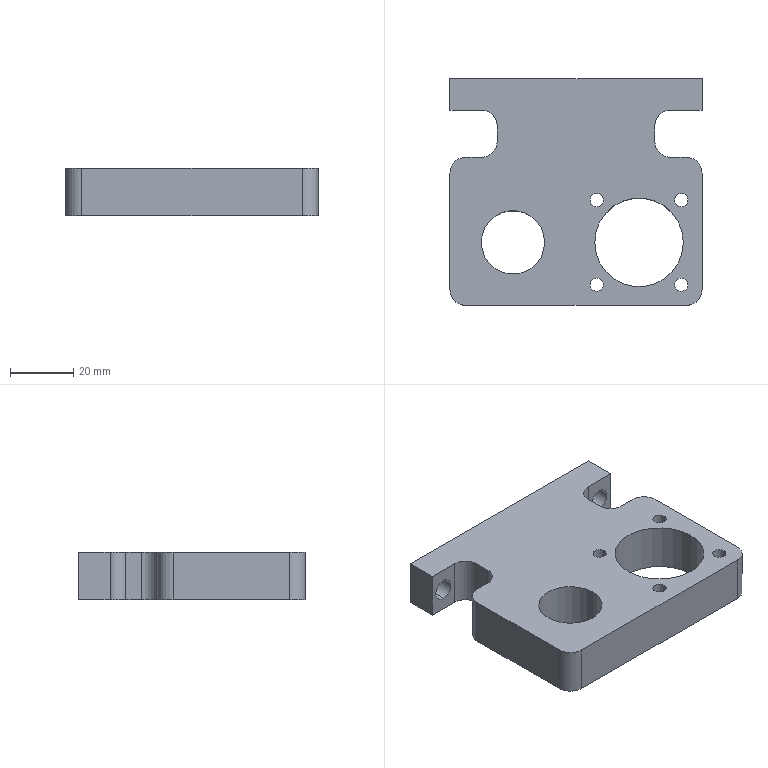Part | SolidWorks | features ICE 2, Extrusion 1, Fillet 1, HoleWzd 1, MoveCopyBody 1 | 1 solid | 38 faces | box 80 x 72 x 15 mm | volume 64030 mm3 | cylinder 24 | plane 14 | commonest cylinder face diameters 4.2 x8 10 x8 6.8 x4 20.1 x2 28.1 x2
STEP:
#1=CARTESIAN_POINT('',(31.335,21.435,7.5));
#2=VERTEX_POINT('',#1);
#3=CARTESIAN_POINT('',(35.535,21.435,7.5));
#4=VERTEX_POINT('',#3);
#5=CARTESIAN_POINT('',(33.435,21.435,7.5));
#6=DIRECTION('',(0.,0.,-1.));
#7=DIRECTION('',(1.,0.,0.));
#8=AXIS2_PLACEMENT_3D('',#5,#6,#7);
#9=CIRCLE('',#8,2.1);
#10=EDGE_CURVE('',#2,#4,#9,.T.);
#11=ORIENTED_EDGE('',*,*,#10,.F.);
#12=CARTESIAN_POINT('',(31.335,21.435,-7.5));
#13=VERTEX_POINT('',#12);
#14=CARTESIAN_POINT('',(31.335,21.435,-7.5));
#15=DIRECTION('',(0.,0.,-1.));
#16=VECTOR('',#15,1000.);
#17=LINE('',#14,#16);
#18=EDGE_CURVE('',#2,#13,#17,.T.);
#19=ORIENTED_EDGE('',*,*,#18,.T.);
#20=CARTESIAN_POINT('',(35.535,21.435,-7.5));
#21=VERTEX_POINT('',#20);
#22=CARTESIAN_POINT('',(33.435,21.435,-7.5));
#23=DIRECTION('',(0.,0.,-1.));
#24=DIRECTION('',(1.,0.,0.));
#25=AXIS2_PLACEMENT_3D('',#22,#23,#24);
#26=CIRCLE('',#25,2.1);
#27=EDGE_CURVE('',#13,#21,#26,.T.);
#28=ORIENTED_EDGE('',*,*,#27,.T.);
#29=CARTESIAN_POINT('',(35.535,21.435,-7.5));
#30=DIRECTION('',(0.,0.,-1.));
#31=VECTOR('',#30,1000.);
#32=LINE('',#29,#31);
#33=EDGE_CURVE('',#4,#21,#32,.T.);
#34=ORIENTED_EDGE('',*,*,#33,.F.);
#35=EDGE_LOOP('',(#11,#19,#28,#34));
#36=FACE_OUTER_BOUND('',#35,.T.);
#37=CARTESIAN_POINT('',(33.435,21.435,-7.5));
#38=DIRECTION('',(0.,0.,-1.));
#39=DIRECTION('',(1.,0.,0.));
#40=AXIS2_PLACEMENT_3D('',#37,#38,#39);
#41=CYLINDRICAL_SURFACE('',#40,2.1);
#42=ADVANCED_FACE('',(#36),#41,.F.);
#43=CARTESIAN_POINT('',(4.465,21.435,7.5));
#44=VERTEX_POINT('',#43);
#45=CARTESIAN_POINT('',(8.665,21.435,7.5));
#46=VERTEX_POINT('',#45);
#47=CARTESIAN_POINT('',(6.565,21.435,7.5));
#48=DIRECTION('',(0.,0.,-1.));
#49=DIRECTION('',(1.,0.,0.));
#50=AXIS2_PLACEMENT_3D('',#47,#48,#49);
#51=CIRCLE('',#50,2.1);
#52=EDGE_CURVE('',#44,#46,#51,.T.);
#53=ORIENTED_EDGE('',*,*,#52,.F.);
#54=CARTESIAN_POINT('',(4.465,21.435,-7.5));
#55=VERTEX_POINT('',#54);
#56=CARTESIAN_POINT('',(4.465,21.435,-7.5));
#57=DIRECTION('',(0.,0.,-1.));
#58=VECTOR('',#57,1000.);
#59=LINE('',#56,#58);
#60=EDGE_CURVE('',#44,#55,#59,.T.);
#61=ORIENTED_EDGE('',*,*,#60,.T.);
#62=CARTESIAN_POINT('',(8.665,21.435,-7.5));
#63=VERTEX_POINT('',#62);
#64=CARTESIAN_POINT('',(6.565,21.435,-7.5));
#65=DIRECTION('',(0.,0.,-1.));
#66=DIRECTION('',(1.,0.,0.));
#67=AXIS2_PLACEMENT_3D('',#64,#65,#66);
#68=CIRCLE('',#67,2.1);
#69=EDGE_CURVE('',#55,#63,#68,.T.);
#70=ORIENTED_EDGE('',*,*,#69,.T.);
#71=CARTESIAN_POINT('',(8.665,21.435,-7.5));
#72=DIRECTION('',(0.,0.,-1.));
#73=VECTOR('',#72,1000.);
#74=LINE('',#71,#73);
#75=EDGE_CURVE('',#46,#63,#74,.T.);
#76=ORIENTED_EDGE('',*,*,#75,.F.);
#77=EDGE_LOOP('',(#53,#61,#70,#76));
#78=FACE_OUTER_BOUND('',#77,.T.);
#79=CARTESIAN_POINT('',(6.565,21.435,-7.5));
#80=DIRECTION('',(0.,0.,-1.));
#81=DIRECTION('',(1.,0.,0.));
#82=AXIS2_PLACEMENT_3D('',#79,#80,#81);
#83=CYLINDRICAL_SURFACE('',#82,2.1);
#84=ADVANCED_FACE('',(#78),#83,.F.);
#85=CARTESIAN_POINT('',(4.465,-5.435,7.5));
#86=VERTEX_POINT('',#85);
#87=CARTESIAN_POINT('',(8.665,-5.435,7.5));
#88=VERTEX_POINT('',#87);
#89=CARTESIAN_POINT('',(6.565,-5.435,7.5));
#90=DIRECTION('',(0.,0.,-1.));
#91=DIRECTION('',(1.,0.,0.));
#92=AXIS2_PLACEMENT_3D('',#89,#90,#91);
#93=CIRCLE('',#92,2.1);
#94=EDGE_CURVE('',#86,#88,#93,.T.);
#95=ORIENTED_EDGE('',*,*,#94,.F.);
#96=CARTESIAN_POINT('',(4.465,-5.435,-7.5));
#97=VERTEX_POINT('',#96);
#98=CARTESIAN_POINT('',(4.465,-5.435,-7.5));
#99=DIRECTION('',(0.,0.,-1.));
#100=VECTOR('',#99,1000.);
#101=LINE('',#98,#100);
#102=EDGE_CURVE('',#86,#97,#101,.T.);
#103=ORIENTED_EDGE('',*,*,#102,.T.);
#104=CARTESIAN_POINT('',(8.665,-5.435,-7.5));
#105=VERTEX_POINT('',#104);
#106=CARTESIAN_POINT('',(6.565,-5.435,-7.5));
#107=DIRECTION('',(0.,0.,-1.));
#108=DIRECTION('',(1.,0.,0.));
#109=AXIS2_PLACEMENT_3D('',#106,#107,#108);
#110=CIRCLE('',#109,2.1);
#111=EDGE_CURVE('',#97,#105,#110,.T.);
#112=ORIENTED_EDGE('',*,*,#111,.T.);
#113=CARTESIAN_POINT('',(8.665,-5.435,-7.5));
#114=DIRECTION('',(0.,0.,-1.));
#115=VECTOR('',#114,1000.);
#116=LINE('',#113,#115);
#117=EDGE_CURVE('',#88,#105,#116,.T.);
#118=ORIENTED_EDGE('',*,*,#117,.F.);
#119=EDGE_LOOP('',(#95,#103,#112,#118));
#120=FACE_OUTER_BOUND('',#119,.T.);
#121=CARTESIAN_POINT('',(6.565,-5.435,-7.5));
#122=DIRECTION('',(0.,0.,-1.));
#123=DIRECTION('',(1.,0.,0.));
#124=AXIS2_PLACEMENT_3D('',#121,#122,#123);
#125=CYLINDRICAL_SURFACE('',#124,2.1);
#126=ADVANCED_FACE('',(#120),#125,.F.);
#127=CARTESIAN_POINT('',(31.335,-5.435,7.5));
#128=VERTEX_POINT('',#127);
#129=CARTESIAN_POINT('',(35.535,-5.435,7.5));
#130=VERTEX_POINT('',#129);
#131=CARTESIAN_POINT('',(33.435,-5.435,7.5));
#132=DIRECTION('',(0.,0.,-1.));
#133=DIRECTION('',(1.,0.,0.));
#134=AXIS2_PLACEMENT_3D('',#131,#132,#133);
#135=CIRCLE('',#134,2.1);
#136=EDGE_CURVE('',#128,#130,#135,.T.);
#137=ORIENTED_EDGE('',*,*,#136,.F.);
#138=CARTESIAN_POINT('',(31.335,-5.435,-7.5));
#139=VERTEX_POINT('',#138);
#140=CARTESIAN_POINT('',(31.335,-5.435,-7.5));
#141=DIRECTION('',(0.,0.,-1.));
#142=VECTOR('',#141,1000.);
#143=LINE('',#140,#142);
#144=EDGE_CURVE('',#128,#139,#143,.T.);
#145=ORIENTED_EDGE('',*,*,#144,.T.);
#146=CARTESIAN_POINT('',(35.535,-5.435,-7.5));
#147=VERTEX_POINT('',#146);
#148=CARTESIAN_POINT('',(33.435,-5.435,-7.5));
#149=DIRECTION('',(0.,0.,-1.));
#150=DIRECTION('',(1.,0.,0.));
#151=AXIS2_PLACEMENT_3D('',#148,#149,#150);
#152=CIRCLE('',#151,2.1);
#153=EDGE_CURVE('',#139,#147,#152,.T.);
#154=ORIENTED_EDGE('',*,*,#153,.T.);
#155=CARTESIAN_POINT('',(35.535,-5.435,-7.5));
#156=DIRECTION('',(0.,0.,-1.));
#157=VECTOR('',#156,1000.);
#158=LINE('',#155,#157);
#159=EDGE_CURVE('',#130,#147,#158,.T.);
#160=ORIENTED_EDGE('',*,*,#159,.F.);
#161=EDGE_LOOP('',(#137,#145,#154,#160));
#162=FACE_OUTER_BOUND('',#161,.T.);
#163=CARTESIAN_POINT('',(33.435,-5.435,-7.5));
#164=DIRECTION('',(0.,0.,-1.));
#165=DIRECTION('',(1.,0.,0.));
#166=AXIS2_PLACEMENT_3D('',#163,#164,#165);
#167=CYLINDRICAL_SURFACE('',#166,2.1);
#168=ADVANCED_FACE('',(#162),#167,.F.);
#169=CARTESIAN_POINT('',(34.05,8.,-7.5));
#170=VERTEX_POINT('',#169);
#171=CARTESIAN_POINT('',(5.95,8.,-7.5));
#172=VERTEX_POINT('',#171);
#173=CARTESIAN_POINT('',(20.,8.,-7.5));
#174=DIRECTION('',(0.,0.,1.));
#175=DIRECTION('',(-1.,0.,0.));
#176=AXIS2_PLACEMENT_3D('',#173,#174,#175);
#177=CIRCLE('',#176,14.05);
#178=EDGE_CURVE('',#170,#172,#177,.T.);
#179=ORIENTED_EDGE('',*,*,#178,.F.);
#180=CARTESIAN_POINT('',(34.05,8.,7.5));
#181=VERTEX_POINT('',#180);
#182=CARTESIAN_POINT('',(34.05,8.,-7.5));
#183=DIRECTION('',(0.,0.,1.));
#184=VECTOR('',#183,1000.);
#185=LINE('',#182,#184);
#186=EDGE_CURVE('',#170,#181,#185,.T.);
#187=ORIENTED_EDGE('',*,*,#186,.T.);
#188=CARTESIAN_POINT('',(5.95,8.,7.5));
#189=VERTEX_POINT('',#188);
#190=CARTESIAN_POINT('',(20.,8.,7.5));
#191=DIRECTION('',(0.,0.,1.));
#192=DIRECTION('',(-1.,0.,0.));
#193=AXIS2_PLACEMENT_3D('',#190,#191,#192);
#194=CIRCLE('',#193,14.05);
#195=EDGE_CURVE('',#181,#189,#194,.T.);
#196=ORIENTED_EDGE('',*,*,#195,.T.);
#197=CARTESIAN_POINT('',(5.95,8.,-7.5));
#198=DIRECTION('',(0.,0.,1.));
#199=VECTOR('',#198,1000.);
#200=LINE('',#197,#199);
#201=EDGE_CURVE('',#172,#189,#200,.T.);
#202=ORIENTED_EDGE('',*,*,#201,.F.);
#203=EDGE_LOOP('',(#179,#187,#196,#202));
#204=FACE_OUTER_BOUND('',#203,.T.);
#205=CARTESIAN_POINT('',(20.,8.,-7.5));
#206=DIRECTION('',(0.,0.,1.));
#207=DIRECTION('',(-1.,0.,0.));
#208=AXIS2_PLACEMENT_3D('',#205,#206,#207);
#209=CYLINDRICAL_SURFACE('',#208,14.05);
#210=ADVANCED_FACE('',(#204),#209,.F.);
#211=CARTESIAN_POINT('',(-9.95,8.,-7.5));
#212=VERTEX_POINT('',#211);
#213=CARTESIAN_POINT('',(-30.05,8.,-7.5));
#214=VERTEX_POINT('',#213);
#215=CARTESIAN_POINT('',(-20.,8.,-7.5));
#216=DIRECTION('',(0.,0.,1.));
#217=DIRECTION('',(-1.,0.,0.));
#218=AXIS2_PLACEMENT_3D('',#215,#216,#217);
#219=CIRCLE('',#218,10.05);
#220=EDGE_CURVE('',#212,#214,#219,.T.);
#221=ORIENTED_EDGE('',*,*,#220,.F.);
#222=CARTESIAN_POINT('',(-9.95,8.,7.5));
#223=VERTEX_POINT('',#222);
#224=CARTESIAN_POINT('',(-9.95,8.,-7.5));
#225=DIRECTION('',(0.,0.,1.));
#226=VECTOR('',#225,1000.);
#227=LINE('',#224,#226);
#228=EDGE_CURVE('',#212,#223,#227,.T.);
#229=ORIENTED_EDGE('',*,*,#228,.T.);
#230=CARTESIAN_POINT('',(-30.05,8.,7.5));
#231=VERTEX_POINT('',#230);
#232=CARTESIAN_POINT('',(-20.,8.,7.5));
#233=DIRECTION('',(0.,0.,1.));
#234=DIRECTION('',(-1.,0.,0.));
#235=AXIS2_PLACEMENT_3D('',#232,#233,#234);
#236=CIRCLE('',#235,10.05);
#237=EDGE_CURVE('',#223,#231,#236,.T.);
#238=ORIENTED_EDGE('',*,*,#237,.T.);
#239=CARTESIAN_POINT('',(-30.05,8.,-7.5));
#240=DIRECTION('',(0.,0.,1.));
#241=VECTOR('',#240,1000.);
#242=LINE('',#239,#241);
#243=EDGE_CURVE('',#214,#231,#242,.T.);
#244=ORIENTED_EDGE('',*,*,#243,.F.);
#245=EDGE_LOOP('',(#221,#229,#238,#244));
#246=FACE_OUTER_BOUND('',#245,.T.);
#247=CARTESIAN_POINT('',(-20.,8.,-7.5));
#248=DIRECTION('',(0.,0.,1.));
#249=DIRECTION('',(-1.,0.,0.));
#250=AXIS2_PLACEMENT_3D('',#247,#248,#249);
#251=CYLINDRICAL_SURFACE('',#250,10.05);
#252=ADVANCED_FACE('',(#246),#251,.F.);
#253=CARTESIAN_POINT('',(-35.,50.,-3.4));
#254=VERTEX_POINT('',#253);
#255=CARTESIAN_POINT('',(-35.,50.,3.4));
#256=VERTEX_POINT('',#255);
#257=CARTESIAN_POINT('',(-35.,50.,0.));
#258=DIRECTION('',(0.,-1.,0.));
#259=DIRECTION('',(0.,0.,-1.));
#260=AXIS2_PLACEMENT_3D('',#257,#258,#259);
#261=CIRCLE('',#260,3.4);
#262=EDGE_CURVE('',#254,#256,#261,.T.);
#263=ORIENTED_EDGE('',*,*,#262,.T.);
#264=CARTESIAN_POINT('',(-35.,60.,3.4));
#265=VERTEX_POINT('',#264);
#266=CARTESIAN_POINT('',(-35.,-12.001,3.4));
#267=DIRECTION('',(0.,1.,0.));
#268=VECTOR('',#267,1000.);
#269=LINE('',#266,#268);
#270=EDGE_CURVE('',#256,#265,#269,.T.);
#271=ORIENTED_EDGE('',*,*,#270,.T.);
#272=CARTESIAN_POINT('',(-35.,60.,-3.4));
#273=VERTEX_POINT('',#272);
#274=CARTESIAN_POINT('',(-35.,60.,0.));
#275=DIRECTION('',(0.,1.,0.));
#276=DIRECTION('',(0.,0.,1.));
#277=AXIS2_PLACEMENT_3D('',#274,#275,#276);
#278=CIRCLE('',#277,3.4);
#279=EDGE_CURVE('',#265,#273,#278,.T.);
#280=ORIENTED_EDGE('',*,*,#279,.T.);
#281=CARTESIAN_POINT('',(-35.,-12.001,-3.4));
#282=DIRECTION('',(0.,1.,0.));
#283=VECTOR('',#282,1000.);
#284=LINE('',#281,#283);
#285=EDGE_CURVE('',#254,#273,#284,.T.);
#286=ORIENTED_EDGE('',*,*,#285,.F.);
#287=EDGE_LOOP('',(#263,#271,#280,#286));
#288=FACE_OUTER_BOUND('',#287,.T.);
#289=CARTESIAN_POINT('',(-35.,-12.001,0.));
#290=DIRECTION('',(0.,1.,0.));
#291=DIRECTION('',(0.,0.,-1.));
#292=AXIS2_PLACEMENT_3D('',#289,#290,#291);
#293=CYLINDRICAL_SURFACE('',#292,3.4);
#294=ADVANCED_FACE('',(#288),#293,.F.);
#295=CARTESIAN_POINT('',(35.,50.,-3.4));
#296=VERTEX_POINT('',#295);
#297=CARTESIAN_POINT('',(35.,50.,3.4));
#298=VERTEX_POINT('',#297);
#299=CARTESIAN_POINT('',(35.,50.,0.));
#300=DIRECTION('',(0.,-1.,0.));
#301=DIRECTION('',(0.,0.,-1.));
#302=AXIS2_PLACEMENT_3D('',#299,#300,#301);
#303=CIRCLE('',#302,3.4);
#304=EDGE_CURVE('',#296,#298,#303,.T.);
#305=ORIENTED_EDGE('',*,*,#304,.T.);
#306=CARTESIAN_POINT('',(35.,60.,3.4));
#307=VERTEX_POINT('',#306);
#308=CARTESIAN_POINT('',(35.,-12.001,3.4));
#309=DIRECTION('',(0.,1.,0.));
#310=VECTOR('',#309,1000.);
#311=LINE('',#308,#310);
#312=EDGE_CURVE('',#298,#307,#311,.T.);
#313=ORIENTED_EDGE('',*,*,#312,.T.);
#314=CARTESIAN_POINT('',(35.,60.,-3.4));
#315=VERTEX_POINT('',#314);
#316=CARTESIAN_POINT('',(35.,60.,0.));
#317=DIRECTION('',(0.,1.,0.));
#318=DIRECTION('',(0.,0.,-1.));
#319=AXIS2_PLACEMENT_3D('',#316,#317,#318);
#320=CIRCLE('',#319,3.4);
#321=EDGE_CURVE('',#307,#315,#320,.T.);
#322=ORIENTED_EDGE('',*,*,#321,.T.);
#323=CARTESIAN_POINT('',(35.,-12.001,-3.4));
#324=DIRECTION('',(0.,1.,0.));
#325=VECTOR('',#324,1000.);
#326=LINE('',#323,#325);
#327=EDGE_CURVE('',#296,#315,#326,.T.);
#328=ORIENTED_EDGE('',*,*,#327,.F.);
#329=EDGE_LOOP('',(#305,#313,#322,#328));
#330=FACE_OUTER_BOUND('',#329,.T.);
#331=CARTESIAN_POINT('',(35.,-12.001,0.));
#332=DIRECTION('',(0.,1.,0.));
#333=DIRECTION('',(0.,0.,-1.));
#334=AXIS2_PLACEMENT_3D('',#331,#332,#333);
#335=CYLINDRICAL_SURFACE('',#334,3.4);
#336=ADVANCED_FACE('',(#330),#335,.F.);
#337=CARTESIAN_POINT('',(40.,50.,-7.5));
#338=VERTEX_POINT('',#337);
#339=CARTESIAN_POINT('',(40.,60.,-7.5));
#340=VERTEX_POINT('',#339);
#341=CARTESIAN_POINT('',(40.,60.,-7.5));
#342=DIRECTION('',(0.,1.,0.));
#343=VECTOR('',#342,1000.);
#344=LINE('',#341,#343);
#345=EDGE_CURVE('',#338,#340,#344,.T.);
#346=ORIENTED_EDGE('',*,*,#345,.T.);
#347=CARTESIAN_POINT('',(40.,60.,7.5));
#348=VERTEX_POINT('',#347);
#349=CARTESIAN_POINT('',(40.,60.,7.5));
#350=DIRECTION('',(0.,0.,-1.));
#351=VECTOR('',#350,1000.);
#352=LINE('',#349,#351);
#353=EDGE_CURVE('',#348,#340,#352,.T.);
#354=ORIENTED_EDGE('',*,*,#353,.F.);
#355=CARTESIAN_POINT('',(40.,50.,7.5));
#356=VERTEX_POINT('',#355);
#357=CARTESIAN_POINT('',(40.,60.,7.5));
#358=DIRECTION('',(0.,1.,0.));
#359=VECTOR('',#358,1000.);
#360=LINE('',#357,#359);
#361=EDGE_CURVE('',#356,#348,#360,.T.);
#362=ORIENTED_EDGE('',*,*,#361,.F.);
#363=CARTESIAN_POINT('',(40.,50.,7.5));
#364=DIRECTION('',(0.,0.,-1.));
#365=VECTOR('',#364,1000.);
#366=LINE('',#363,#365);
#367=EDGE_CURVE('',#356,#338,#366,.T.);
#368=ORIENTED_EDGE('',*,*,#367,.T.);
#369=EDGE_LOOP('',(#346,#354,#362,#368));
#370=FACE_OUTER_BOUND('',#369,.T.);
#371=CARTESIAN_POINT('',(40.,60.,7.5));
#372=DIRECTION('',(-1.,0.,0.));
#373=DIRECTION('',(0.,0.,-1.));
#374=AXIS2_PLACEMENT_3D('',#371,#372,#373);
#375=PLANE('',#374);
#376=ADVANCED_FACE('',(#370),#375,.F.);
#377=CARTESIAN_POINT('',(35.,60.,0.));
#378=DIRECTION('',(0.,1.,0.));
#379=DIRECTION('',(0.,0.,-1.));
#380=AXIS2_PLACEMENT_3D('',#377,#378,#379);
#381=CIRCLE('',#380,3.4);
#382=EDGE_CURVE('',#315,#307,#381,.T.);
#383=ORIENTED_EDGE('',*,*,#382,.F.);
#384=ORIENTED_EDGE('',*,*,#321,.F.);
#385=EDGE_LOOP('',(#383,#384));
#386=FACE_BOUND('',#385,.T.);
#387=CARTESIAN_POINT('',(-35.,60.,0.));
#388=DIRECTION('',(0.,1.,0.));
#389=DIRECTION('',(0.,0.,1.));
#390=AXIS2_PLACEMENT_3D('',#387,#388,#389);
#391=CIRCLE('',#390,3.4);
#392=EDGE_CURVE('',#273,#265,#391,.T.);
#393=ORIENTED_EDGE('',*,*,#392,.F.);
#394=ORIENTED_EDGE('',*,*,#279,.F.);
#395=EDGE_LOOP('',(#393,#394));
#396=FACE_BOUND('',#395,.T.);
#397=CARTESIAN_POINT('',(-40.,60.,-7.5));
#398=VERTEX_POINT('',#397);
#399=CARTESIAN_POINT('',(-40.,60.,-7.5));
#400=DIRECTION('',(-1.,0.,0.));
#401=VECTOR('',#400,1000.);
#402=LINE('',#399,#401);
#403=EDGE_CURVE('',#340,#398,#402,.T.);
#404=ORIENTED_EDGE('',*,*,#403,.T.);
#405=CARTESIAN_POINT('',(-40.,60.,7.5));
#406=VERTEX_POINT('',#405);
#407=CARTESIAN_POINT('',(-40.,60.,7.5));
#408=DIRECTION('',(0.,0.,-1.));
#409=VECTOR('',#408,1000.);
#410=LINE('',#407,#409);
#411=EDGE_CURVE('',#406,#398,#410,.T.);
#412=ORIENTED_EDGE('',*,*,#411,.F.);
#413=CARTESIAN_POINT('',(-40.,60.,7.5));
#414=DIRECTION('',(-1.,0.,0.));
#415=VECTOR('',#414,1000.);
#416=LINE('',#413,#415);
#417=EDGE_CURVE('',#348,#406,#416,.T.);
#418=ORIENTED_EDGE('',*,*,#417,.F.);
#419=ORIENTED_EDGE('',*,*,#353,.T.);
#420=EDGE_LOOP('',(#404,#412,#418,#419));
#421=FACE_OUTER_BOUND('',#420,.T.);
#422=CARTESIAN_POINT('',(-40.,60.,7.5));
#423=DIRECTION('',(0.,-1.,0.));
#424=DIRECTION('',(0.,0.,1.));
#425=AXIS2_PLACEMENT_3D('',#422,#423,#424);
#426=PLANE('',#425);
#427=ADVANCED_FACE('',(#386,#396,#421),#426,.F.);
#428=CARTESIAN_POINT('',(-40.,50.,-7.5));
#429=VERTEX_POINT('',#428);
#430=CARTESIAN_POINT('',(-40.,60.,-7.5));
#431=DIRECTION('',(0.,-1.,0.));
#432=VECTOR('',#431,1000.);
#433=LINE('',#430,#432);
#434=EDGE_CURVE('',#398,#429,#433,.T.);
#435=ORIENTED_EDGE('',*,*,#434,.T.);
#436=CARTESIAN_POINT('',(-40.,50.,7.5));
#437=VERTEX_POINT('',#436);
#438=CARTESIAN_POINT('',(-40.,50.,7.5));
#439=DIRECTION('',(0.,0.,-1.));
#440=VECTOR('',#439,1000.);
#441=LINE('',#438,#440);
#442=EDGE_CURVE('',#437,#429,#441,.T.);
#443=ORIENTED_EDGE('',*,*,#442,.F.);
#444=CARTESIAN_POINT('',(-40.,60.,7.5));
#445=DIRECTION('',(0.,-1.,0.));
#446=VECTOR('',#445,1000.);
#447=LINE('',#444,#446);
#448=EDGE_CURVE('',#406,#437,#447,.T.);
#449=ORIENTED_EDGE('',*,*,#448,.F.);
#450=ORIENTED_EDGE('',*,*,#411,.T.);
#451=EDGE_LOOP('',(#435,#443,#449,#450));
#452=FACE_OUTER_BOUND('',#451,.T.);
#453=CARTESIAN_POINT('',(-40.,60.,7.5));
#454=DIRECTION('',(1.,0.,0.));
#455=DIRECTION('',(0.,0.,1.));
#456=AXIS2_PLACEMENT_3D('',#453,#454,#455);
#457=PLANE('',#456);
#458=ADVANCED_FACE('',(#452),#457,.F.);
#459=ORIENTED_EDGE('',*,*,#262,.F.);
#460=CARTESIAN_POINT('',(-35.,50.,0.));
#461=DIRECTION('',(0.,-1.,0.));
#462=DIRECTION('',(0.,0.,-1.));
#463=AXIS2_PLACEMENT_3D('',#460,#461,#462);
#464=CIRCLE('',#463,3.4);
#465=EDGE_CURVE('',#256,#254,#464,.T.);
#466=ORIENTED_EDGE('',*,*,#465,.F.);
#467=EDGE_LOOP('',(#459,#466));
#468=FACE_BOUND('',#467,.T.);
#469=CARTESIAN_POINT('',(-30.,50.,-7.5));
#470=VERTEX_POINT('',#469);
#471=CARTESIAN_POINT('',(-40.,50.,-7.5));
#472=DIRECTION('',(1.,0.,0.));
#473=VECTOR('',#472,1000.);
#474=LINE('',#471,#473);
#475=EDGE_CURVE('',#429,#470,#474,.T.);
#476=ORIENTED_EDGE('',*,*,#475,.T.);
#477=CARTESIAN_POINT('',(-30.,50.,7.5));
#478=VERTEX_POINT('',#477);
#479=CARTESIAN_POINT('',(-30.,50.,7.5));
#480=DIRECTION('',(0.,0.,1.));
#481=VECTOR('',#480,1000.);
#482=LINE('',#479,#481);
#483=EDGE_CURVE('',#470,#478,#482,.T.);
#484=ORIENTED_EDGE('',*,*,#483,.T.);
#485=CARTESIAN_POINT('',(-40.,50.,7.5));
#486=DIRECTION('',(1.,0.,0.));
#487=VECTOR('',#486,1000.);
#488=LINE('',#485,#487);
#489=EDGE_CURVE('',#437,#478,#488,.T.);
#490=ORIENTED_EDGE('',*,*,#489,.F.);
#491=ORIENTED_EDGE('',*,*,#442,.T.);
#492=EDGE_LOOP('',(#476,#484,#490,#491));
#493=FACE_OUTER_BOUND('',#492,.T.);
#494=CARTESIAN_POINT('',(-40.,50.,7.5));
#495=DIRECTION('',(0.,1.,0.));
#496=DIRECTION('',(0.,0.,-1.));
#497=AXIS2_PLACEMENT_3D('',#494,#495,#496);
#498=PLANE('',#497);
#499=ADVANCED_FACE('',(#468,#493),#498,.F.);
#500=CARTESIAN_POINT('',(-25.,45.,-7.5));
#501=VERTEX_POINT('',#500);
#502=CARTESIAN_POINT('',(-25.,40.,-7.5));
#503=VERTEX_POINT('',#502);
#504=CARTESIAN_POINT('',(-25.,50.,-7.5));
#505=DIRECTION('',(0.,-1.,0.));
#506=VECTOR('',#505,1000.);
#507=LINE('',#504,#506);
#508=EDGE_CURVE('',#501,#503,#507,.T.);
#509=ORIENTED_EDGE('',*,*,#508,.T.);
#510=CARTESIAN_POINT('',(-25.,40.,7.5));
#511=VERTEX_POINT('',#510);
#512=CARTESIAN_POINT('',(-25.,40.,7.5));
#513=DIRECTION('',(0.,0.,1.));
#514=VECTOR('',#513,1000.);
#515=LINE('',#512,#514);
#516=EDGE_CURVE('',#503,#511,#515,.T.);
#517=ORIENTED_EDGE('',*,*,#516,.T.);
#518=CARTESIAN_POINT('',(-25.,45.,7.5));
#519=VERTEX_POINT('',#518);
#520=CARTESIAN_POINT('',(-25.,50.,7.5));
#521=DIRECTION('',(0.,-1.,0.));
#522=VECTOR('',#521,1000.);
#523=LINE('',#520,#522);
#524=EDGE_CURVE('',#519,#511,#523,.T.);
#525=ORIENTED_EDGE('',*,*,#524,.F.);
#526=CARTESIAN_POINT('',(-25.,45.,-7.5));
#527=DIRECTION('',(0.,0.,-1.));
#528=VECTOR('',#527,1000.);
#529=LINE('',#526,#528);
#530=EDGE_CURVE('',#519,#501,#529,.T.);
#531=ORIENTED_EDGE('',*,*,#530,.T.);
#532=EDGE_LOOP('',(#509,#517,#525,#531));
#533=FACE_OUTER_BOUND('',#532,.T.);
#534=CARTESIAN_POINT('',(-25.,50.,7.5));
#535=DIRECTION('',(1.,0.,0.));
#536=DIRECTION('',(0.,0.,1.));
#537=AXIS2_PLACEMENT_3D('',#534,#535,#536);
#538=PLANE('',#537);
#539=ADVANCED_FACE('',(#533),#538,.F.);
#540=CARTESIAN_POINT('',(-30.,35.,-7.5));
#541=VERTEX_POINT('',#540);
#542=CARTESIAN_POINT('',(-35.,35.,-7.5));
#543=VERTEX_POINT('',#542);
#544=CARTESIAN_POINT('',(-25.,35.,-7.5));
#545=DIRECTION('',(-1.,0.,0.));
#546=VECTOR('',#545,1000.);
#547=LINE('',#544,#546);
#548=EDGE_CURVE('',#541,#543,#547,.T.);
#549=ORIENTED_EDGE('',*,*,#548,.T.);
#550=CARTESIAN_POINT('',(-35.,35.,7.5));
#551=VERTEX_POINT('',#550);
#552=CARTESIAN_POINT('',(-35.,35.,7.5));
#553=DIRECTION('',(0.,0.,1.));
#554=VECTOR('',#553,1000.);
#555=LINE('',#552,#554);
#556=EDGE_CURVE('',#543,#551,#555,.T.);
#557=ORIENTED_EDGE('',*,*,#556,.T.);
#558=CARTESIAN_POINT('',(-30.,35.,7.5));
#559=VERTEX_POINT('',#558);
#560=CARTESIAN_POINT('',(-25.,35.,7.5));
#561=DIRECTION('',(-1.,0.,0.));
#562=VECTOR('',#561,1000.);
#563=LINE('',#560,#562);
#564=EDGE_CURVE('',#559,#551,#563,.T.);
#565=ORIENTED_EDGE('',*,*,#564,.F.);
#566=CARTESIAN_POINT('',(-30.,35.,-7.5));
#567=DIRECTION('',(0.,0.,-1.));
#568=VECTOR('',#567,1000.);
#569=LINE('',#566,#568);
#570=EDGE_CURVE('',#559,#541,#569,.T.);
#571=ORIENTED_EDGE('',*,*,#570,.T.);
#572=EDGE_LOOP('',(#549,#557,#565,#571));
#573=FACE_OUTER_BOUND('',#572,.T.);
#574=CARTESIAN_POINT('',(-25.,35.,7.5));
#575=DIRECTION('',(0.,-1.,0.));
#576=DIRECTION('',(0.,0.,1.));
#577=AXIS2_PLACEMENT_3D('',#574,#575,#576);
#578=PLANE('',#577);
#579=ADVANCED_FACE('',(#573),#578,.F.);
#580=CARTESIAN_POINT('',(-40.,30.,-7.5));
#581=VERTEX_POINT('',#580);
#582=CARTESIAN_POINT('',(-40.,-7.,-7.5));
#583=VERTEX_POINT('',#582);
#584=CARTESIAN_POINT('',(-40.,35.,-7.5));
#585=DIRECTION('',(0.,-1.,0.));
#586=VECTOR('',#585,1000.);
#587=LINE('',#584,#586);
#588=EDGE_CURVE('',#581,#583,#587,.T.);
#589=ORIENTED_EDGE('',*,*,#588,.T.);
#590=CARTESIAN_POINT('',(-40.,-7.,7.5));
#591=VERTEX_POINT('',#590);
#592=CARTESIAN_POINT('',(-40.,-7.,7.5));
#593=DIRECTION('',(0.,0.,1.));
#594=VECTOR('',#593,1000.);
#595=LINE('',#592,#594);
#596=EDGE_CURVE('',#583,#591,#595,.T.);
#597=ORIENTED_EDGE('',*,*,#596,.T.);
#598=CARTESIAN_POINT('',(-40.,30.,7.5));
#599=VERTEX_POINT('',#598);
#600=CARTESIAN_POINT('',(-40.,35.,7.5));
#601=DIRECTION('',(0.,-1.,0.));
#602=VECTOR('',#601,1000.);
#603=LINE('',#600,#602);
#604=EDGE_CURVE('',#599,#591,#603,.T.);
#605=ORIENTED_EDGE('',*,*,#604,.F.);
#606=CARTESIAN_POINT('',(-40.,30.,7.5));
#607=DIRECTION('',(0.,0.,-1.));
#608=VECTOR('',#607,1000.);
#609=LINE('',#606,#608);
#610=EDGE_CURVE('',#599,#581,#609,.T.);
#611=ORIENTED_EDGE('',*,*,#610,.T.);
#612=EDGE_LOOP('',(#589,#597,#605,#611));
#613=FACE_OUTER_BOUND('',#612,.T.);
#614=CARTESIAN_POINT('',(-40.,35.,7.5));
#615=DIRECTION('',(1.,0.,0.));
#616=DIRECTION('',(0.,1.,0.));
#617=AXIS2_PLACEMENT_3D('',#614,#615,#616);
#618=PLANE('',#617);
#619=ADVANCED_FACE('',(#613),#618,.F.);
#620=CARTESIAN_POINT('',(-35.,-12.,-7.5));
#621=VERTEX_POINT('',#620);
#622=CARTESIAN_POINT('',(35.,-12.,-7.5));
#623=VERTEX_POINT('',#622);
#624=CARTESIAN_POINT('',(40.,-12.,-7.5));
#625=DIRECTION('',(1.,0.,0.));
#626=VECTOR('',#625,1000.);
#627=LINE('',#624,#626);
#628=EDGE_CURVE('',#621,#623,#627,.T.);
#629=ORIENTED_EDGE('',*,*,#628,.T.);
#630=CARTESIAN_POINT('',(35.,-12.,7.5));
#631=VERTEX_POINT('',#630);
#632=CARTESIAN_POINT('',(35.,-12.,7.5));
#633=DIRECTION('',(0.,0.,1.));
#634=VECTOR('',#633,1000.);
#635=LINE('',#632,#634);
#636=EDGE_CURVE('',#623,#631,#635,.T.);
#637=ORIENTED_EDGE('',*,*,#636,.T.);
#638=CARTESIAN_POINT('',(-35.,-12.,7.5));
#639=VERTEX_POINT('',#638);
#640=CARTESIAN_POINT('',(40.,-12.,7.5));
#641=DIRECTION('',(1.,0.,0.));
#642=VECTOR('',#641,1000.);
#643=LINE('',#640,#642);
#644=EDGE_CURVE('',#639,#631,#643,.T.);
#645=ORIENTED_EDGE('',*,*,#644,.F.);
#646=CARTESIAN_POINT('',(-35.,-12.,7.5));
#647=DIRECTION('',(0.,0.,-1.));
#648=VECTOR('',#647,1000.);
#649=LINE('',#646,#648);
#650=EDGE_CURVE('',#639,#621,#649,.T.);
#651=ORIENTED_EDGE('',*,*,#650,.T.);
#652=EDGE_LOOP('',(#629,#637,#645,#651));
#653=FACE_OUTER_BOUND('',#652,.T.);
#654=CARTESIAN_POINT('',(40.,-12.,7.5));
#655=DIRECTION('',(0.,1.,0.));
#656=DIRECTION('',(0.,0.,-1.));
#657=AXIS2_PLACEMENT_3D('',#654,#655,#656);
#658=PLANE('',#657);
#659=ADVANCED_FACE('',(#653),#658,.F.);
#660=CARTESIAN_POINT('',(40.,-7.,-7.5));
#661=VERTEX_POINT('',#660);
#662=CARTESIAN_POINT('',(40.,30.,-7.5));
#663=VERTEX_POINT('',#662);
#664=CARTESIAN_POINT('',(40.,35.,-7.5));
#665=DIRECTION('',(0.,1.,0.));
#666=VECTOR('',#665,1000.);
#667=LINE('',#664,#666);
#668=EDGE_CURVE('',#661,#663,#667,.T.);
#669=ORIENTED_EDGE('',*,*,#668,.T.);
#670=CARTESIAN_POINT('',(40.,30.,7.5));
#671=VERTEX_POINT('',#670);
#672=CARTESIAN_POINT('',(40.,30.,7.5));
#673=DIRECTION('',(0.,0.,1.));
#674=VECTOR('',#673,1000.);
#675=LINE('',#672,#674);
#676=EDGE_CURVE('',#663,#671,#675,.T.);
#677=ORIENTED_EDGE('',*,*,#676,.T.);
#678=CARTESIAN_POINT('',(40.,-7.,7.5));
#679=VERTEX_POINT('',#678);
#680=CARTESIAN_POINT('',(40.,35.,7.5));
#681=DIRECTION('',(0.,1.,0.));
#682=VECTOR('',#681,1000.);
#683=LINE('',#680,#682);
#684=EDGE_CURVE('',#679,#671,#683,.T.);
#685=ORIENTED_EDGE('',*,*,#684,.F.);
#686=CARTESIAN_POINT('',(40.,-7.,7.5));
#687=DIRECTION('',(0.,0.,-1.));
#688=VECTOR('',#687,1000.);
#689=LINE('',#686,#688);
#690=EDGE_CURVE('',#679,#661,#689,.T.);
#691=ORIENTED_EDGE('',*,*,#690,.T.);
#692=EDGE_LOOP('',(#669,#677,#685,#691));
#693=FACE_OUTER_BOUND('',#692,.T.);
#694=CARTESIAN_POINT('',(40.,35.,7.5));
#695=DIRECTION('',(-1.,0.,0.));
#696=DIRECTION('',(0.,-1.,0.));
#697=AXIS2_PLACEMENT_3D('',#694,#695,#696);
#698=PLANE('',#697);
#699=ADVANCED_FACE('',(#693),#698,.F.);
#700=CARTESIAN_POINT('',(35.,35.,7.5));
#701=VERTEX_POINT('',#700);
#702=CARTESIAN_POINT('',(30.,35.,7.5));
#703=VERTEX_POINT('',#702);
#704=CARTESIAN_POINT('',(25.,35.,7.5));
#705=DIRECTION('',(-1.,0.,0.));
#706=VECTOR('',#705,1000.);
#707=LINE('',#704,#706);
#708=EDGE_CURVE('',#701,#703,#707,.T.);
#709=ORIENTED_EDGE('',*,*,#708,.F.);
#710=CARTESIAN_POINT('',(35.,35.,-7.5));
#711=VERTEX_POINT('',#710);
#712=CARTESIAN_POINT('',(35.,35.,7.5));
#713=DIRECTION('',(0.,0.,-1.));
#714=VECTOR('',#713,1000.);
#715=LINE('',#712,#714);
#716=EDGE_CURVE('',#701,#711,#715,.T.);
#717=ORIENTED_EDGE('',*,*,#716,.T.);
#718=CARTESIAN_POINT('',(30.,35.,-7.5));
#719=VERTEX_POINT('',#718);
#720=CARTESIAN_POINT('',(25.,35.,-7.5));
#721=DIRECTION('',(-1.,0.,0.));
#722=VECTOR('',#721,1000.);
#723=LINE('',#720,#722);
#724=EDGE_CURVE('',#711,#719,#723,.T.);
#725=ORIENTED_EDGE('',*,*,#724,.T.);
#726=CARTESIAN_POINT('',(30.,35.,7.5));
#727=DIRECTION('',(0.,0.,1.));
#728=VECTOR('',#727,1000.);
#729=LINE('',#726,#728);
#730=EDGE_CURVE('',#719,#703,#729,.T.);
#731=ORIENTED_EDGE('',*,*,#730,.T.);
#732=EDGE_LOOP('',(#709,#717,#725,#731));
#733=FACE_OUTER_BOUND('',#732,.T.);
#734=CARTESIAN_POINT('',(25.,35.,7.5));
#735=DIRECTION('',(0.,-1.,0.));
#736=DIRECTION('',(0.,0.,1.));
#737=AXIS2_PLACEMENT_3D('',#734,#735,#736);
#738=PLANE('',#737);
#739=ADVANCED_FACE('',(#733),#738,.F.);
#740=CARTESIAN_POINT('',(25.,40.,-7.5));
#741=VERTEX_POINT('',#740);
#742=CARTESIAN_POINT('',(25.,45.,-7.5));
#743=VERTEX_POINT('',#742);
#744=CARTESIAN_POINT('',(25.,50.,-7.5));
#745=DIRECTION('',(0.,1.,0.));
#746=VECTOR('',#745,1000.);
#747=LINE('',#744,#746);
#748=EDGE_CURVE('',#741,#743,#747,.T.);
#749=ORIENTED_EDGE('',*,*,#748,.T.);
#750=CARTESIAN_POINT('',(25.,45.,7.5));
#751=VERTEX_POINT('',#750);
#752=CARTESIAN_POINT('',(25.,45.,7.5));
#753=DIRECTION('',(0.,0.,1.));
#754=VECTOR('',#753,1000.);
#755=LINE('',#752,#754);
#756=EDGE_CURVE('',#743,#751,#755,.T.);
#757=ORIENTED_EDGE('',*,*,#756,.T.);
#758=CARTESIAN_POINT('',(25.,40.,7.5));
#759=VERTEX_POINT('',#758);
#760=CARTESIAN_POINT('',(25.,50.,7.5));
#761=DIRECTION('',(0.,1.,0.));
#762=VECTOR('',#761,1000.);
#763=LINE('',#760,#762);
#764=EDGE_CURVE('',#759,#751,#763,.T.);
#765=ORIENTED_EDGE('',*,*,#764,.F.);
#766=CARTESIAN_POINT('',(25.,40.,-7.5));
#767=DIRECTION('',(0.,0.,-1.));
#768=VECTOR('',#767,1000.);
#769=LINE('',#766,#768);
#770=EDGE_CURVE('',#759,#741,#769,.T.);
#771=ORIENTED_EDGE('',*,*,#770,.T.);
#772=EDGE_LOOP('',(#749,#757,#765,#771));
#773=FACE_OUTER_BOUND('',#772,.T.);
#774=CARTESIAN_POINT('',(25.,50.,7.5));
#775=DIRECTION('',(-1.,0.,0.));
#776=DIRECTION('',(0.,0.,-1.));
#777=AXIS2_PLACEMENT_3D('',#774,#775,#776);
#778=PLANE('',#777);
#779=ADVANCED_FACE('',(#773),#778,.F.);
#780=ORIENTED_EDGE('',*,*,#304,.F.);
#781=CARTESIAN_POINT('',(35.,50.,0.));
#782=DIRECTION('',(0.,-1.,0.));
#783=DIRECTION('',(0.,0.,-1.));
#784=AXIS2_PLACEMENT_3D('',#781,#782,#783);
#785=CIRCLE('',#784,3.4);
#786=EDGE_CURVE('',#298,#296,#785,.T.);
#787=ORIENTED_EDGE('',*,*,#786,.F.);
#788=EDGE_LOOP('',(#780,#787));
#789=FACE_BOUND('',#788,.T.);
#790=CARTESIAN_POINT('',(30.,50.,7.5));
#791=VERTEX_POINT('',#790);
#792=CARTESIAN_POINT('',(40.,50.,7.5));
#793=DIRECTION('',(1.,0.,0.));
#794=VECTOR('',#793,1000.);
#795=LINE('',#792,#794);
#796=EDGE_CURVE('',#791,#356,#795,.T.);
#797=ORIENTED_EDGE('',*,*,#796,.F.);
#798=CARTESIAN_POINT('',(30.,50.,-7.5));
#799=VERTEX_POINT('',#798);
#800=CARTESIAN_POINT('',(30.,50.,-7.5));
#801=DIRECTION('',(0.,0.,-1.));
#802=VECTOR('',#801,1000.);
#803=LINE('',#800,#802);
#804=EDGE_CURVE('',#791,#799,#803,.T.);
#805=ORIENTED_EDGE('',*,*,#804,.T.);
#806=CARTESIAN_POINT('',(40.,50.,-7.5));
#807=DIRECTION('',(1.,0.,0.));
#808=VECTOR('',#807,1000.);
#809=LINE('',#806,#808);
#810=EDGE_CURVE('',#799,#338,#809,.T.);
#811=ORIENTED_EDGE('',*,*,#810,.T.);
#812=ORIENTED_EDGE('',*,*,#367,.F.);
#813=EDGE_LOOP('',(#797,#805,#811,#812));
#814=FACE_OUTER_BOUND('',#813,.T.);
#815=CARTESIAN_POINT('',(40.,50.,7.5));
#816=DIRECTION('',(0.,1.,0.));
#817=DIRECTION('',(0.,0.,-1.));
#818=AXIS2_PLACEMENT_3D('',#815,#816,#817);
#819=PLANE('',#818);
#820=ADVANCED_FACE('',(#789,#814),#819,.F.);
#821=CARTESIAN_POINT('',(33.435,21.435,7.5));
#822=DIRECTION('',(0.,0.,-1.));
#823=DIRECTION('',(1.,0.,0.));
#824=AXIS2_PLACEMENT_3D('',#821,#822,#823);
#825=CIRCLE('',#824,2.1);
#826=EDGE_CURVE('',#4,#2,#825,.T.);
#827=ORIENTED_EDGE('',*,*,#826,.T.);
#828=ORIENTED_EDGE('',*,*,#10,.T.);
#829=EDGE_LOOP('',(#827,#828));
#830=FACE_BOUND('',#829,.T.);
#831=CARTESIAN_POINT('',(6.565,21.435,7.5));
#832=DIRECTION('',(0.,0.,-1.));
#833=DIRECTION('',(1.,0.,0.));
#834=AXIS2_PLACEMENT_3D('',#831,#832,#833);
#835=CIRCLE('',#834,2.1);
#836=EDGE_CURVE('',#46,#44,#835,.T.);
#837=ORIENTED_EDGE('',*,*,#836,.T.);
#838=ORIENTED_EDGE('',*,*,#52,.T.);
#839=EDGE_LOOP('',(#837,#838));
#840=FACE_BOUND('',#839,.T.);
#841=CARTESIAN_POINT('',(6.565,-5.435,7.5));
#842=DIRECTION('',(0.,0.,-1.));
#843=DIRECTION('',(1.,0.,0.));
#844=AXIS2_PLACEMENT_3D('',#841,#842,#843);
#845=CIRCLE('',#844,2.1);
#846=EDGE_CURVE('',#88,#86,#845,.T.);
#847=ORIENTED_EDGE('',*,*,#846,.T.);
#848=ORIENTED_EDGE('',*,*,#94,.T.);
#849=EDGE_LOOP('',(#847,#848));
#850=FACE_BOUND('',#849,.T.);
#851=CARTESIAN_POINT('',(33.435,-5.435,7.5));
#852=DIRECTION('',(0.,0.,-1.));
#853=DIRECTION('',(1.,0.,0.));
#854=AXIS2_PLACEMENT_3D('',#851,#852,#853);
#855=CIRCLE('',#854,2.1);
#856=EDGE_CURVE('',#130,#128,#855,.T.);
#857=ORIENTED_EDGE('',*,*,#856,.T.);
#858=ORIENTED_EDGE('',*,*,#136,.T.);
#859=EDGE_LOOP('',(#857,#858));
#860=FACE_BOUND('',#859,.T.);
#861=CARTESIAN_POINT('',(20.,8.,7.5));
#862=DIRECTION('',(0.,0.,1.));
#863=DIRECTION('',(-1.,0.,0.));
#864=AXIS2_PLACEMENT_3D('',#861,#862,#863);
#865=CIRCLE('',#864,14.05);
#866=EDGE_CURVE('',#189,#181,#865,.T.);
#867=ORIENTED_EDGE('',*,*,#866,.F.);
#868=ORIENTED_EDGE('',*,*,#195,.F.);
#869=EDGE_LOOP('',(#867,#868));
#870=FACE_BOUND('',#869,.T.);
#871=CARTESIAN_POINT('',(-20.,8.,7.5));
#872=DIRECTION('',(0.,0.,1.));
#873=DIRECTION('',(-1.,0.,0.));
#874=AXIS2_PLACEMENT_3D('',#871,#872,#873);
#875=CIRCLE('',#874,10.05);
#876=EDGE_CURVE('',#231,#223,#875,.T.);
#877=ORIENTED_EDGE('',*,*,#876,.F.);
#878=ORIENTED_EDGE('',*,*,#237,.F.);
#879=EDGE_LOOP('',(#877,#878));
#880=FACE_BOUND('',#879,.T.);
#881=ORIENTED_EDGE('',*,*,#684,.T.);
#882=CARTESIAN_POINT('',(35.,30.,7.5));
#883=DIRECTION('',(0.,0.,1.));
#884=DIRECTION('',(1.,0.,0.));
#885=AXIS2_PLACEMENT_3D('',#882,#883,#884);
#886=CIRCLE('',#885,5.);
#887=EDGE_CURVE('',#671,#701,#886,.T.);
#888=ORIENTED_EDGE('',*,*,#887,.T.);
#889=ORIENTED_EDGE('',*,*,#708,.T.);
#890=CARTESIAN_POINT('',(30.,40.,7.5));
#891=DIRECTION('',(0.,0.,-1.));
#892=DIRECTION('',(1.,0.,0.));
#893=AXIS2_PLACEMENT_3D('',#890,#891,#892);
#894=CIRCLE('',#893,5.);
#895=EDGE_CURVE('',#703,#759,#894,.T.);
#896=ORIENTED_EDGE('',*,*,#895,.T.);
#897=ORIENTED_EDGE('',*,*,#764,.T.);
#898=CARTESIAN_POINT('',(30.,45.,7.5));
#899=DIRECTION('',(0.,0.,-1.));
#900=DIRECTION('',(1.,0.,0.));
#901=AXIS2_PLACEMENT_3D('',#898,#899,#900);
#902=CIRCLE('',#901,5.);
#903=EDGE_CURVE('',#751,#791,#902,.T.);
#904=ORIENTED_EDGE('',*,*,#903,.T.);
#905=ORIENTED_EDGE('',*,*,#796,.T.);
#906=ORIENTED_EDGE('',*,*,#361,.T.);
#907=ORIENTED_EDGE('',*,*,#417,.T.);
#908=ORIENTED_EDGE('',*,*,#448,.T.);
#909=ORIENTED_EDGE('',*,*,#489,.T.);
#910=CARTESIAN_POINT('',(-30.,45.,7.5));
#911=DIRECTION('',(0.,0.,-1.));
#912=DIRECTION('',(1.,0.,0.));
#913=AXIS2_PLACEMENT_3D('',#910,#911,#912);
#914=CIRCLE('',#913,5.);
#915=EDGE_CURVE('',#478,#519,#914,.T.);
#916=ORIENTED_EDGE('',*,*,#915,.T.);
#917=ORIENTED_EDGE('',*,*,#524,.T.);
#918=CARTESIAN_POINT('',(-30.,40.,7.5));
#919=DIRECTION('',(0.,0.,-1.));
#920=DIRECTION('',(1.,0.,0.));
#921=AXIS2_PLACEMENT_3D('',#918,#919,#920);
#922=CIRCLE('',#921,5.);
#923=EDGE_CURVE('',#511,#559,#922,.T.);
#924=ORIENTED_EDGE('',*,*,#923,.T.);
#925=ORIENTED_EDGE('',*,*,#564,.T.);
#926=CARTESIAN_POINT('',(-35.,30.,7.5));
#927=DIRECTION('',(0.,0.,1.));
#928=DIRECTION('',(1.,0.,0.));
#929=AXIS2_PLACEMENT_3D('',#926,#927,#928);
#930=CIRCLE('',#929,5.);
#931=EDGE_CURVE('',#551,#599,#930,.T.);
#932=ORIENTED_EDGE('',*,*,#931,.T.);
#933=ORIENTED_EDGE('',*,*,#604,.T.);
#934=CARTESIAN_POINT('',(-35.,-7.,7.5));
#935=DIRECTION('',(0.,0.,1.));
#936=DIRECTION('',(1.,0.,0.));
#937=AXIS2_PLACEMENT_3D('',#934,#935,#936);
#938=CIRCLE('',#937,5.);
#939=EDGE_CURVE('',#591,#639,#938,.T.);
#940=ORIENTED_EDGE('',*,*,#939,.T.);
#941=ORIENTED_EDGE('',*,*,#644,.T.);
#942=CARTESIAN_POINT('',(35.,-7.,7.5));
#943=DIRECTION('',(0.,0.,1.));
#944=DIRECTION('',(1.,0.,0.));
#945=AXIS2_PLACEMENT_3D('',#942,#943,#944);
#946=CIRCLE('',#945,5.);
#947=EDGE_CURVE('',#631,#679,#946,.T.);
#948=ORIENTED_EDGE('',*,*,#947,.T.);
#949=EDGE_LOOP('',(#881,#888,#889,#896,#897,#904,#905,#906,#907,#908,#909,#916,#917,#924,#925,#932,#933,#940,#941,#948));
#950=FACE_OUTER_BOUND('',#949,.T.);
#951=CARTESIAN_POINT('',(0.,60.,7.5));
#952=DIRECTION('',(0.,0.,-1.));
#953=DIRECTION('',(1.,0.,0.));
#954=AXIS2_PLACEMENT_3D('',#951,#952,#953);
#955=PLANE('',#954);
#956=ADVANCED_FACE('',(#830,#840,#850,#860,#870,#880,#950),#955,.F.);
#957=CARTESIAN_POINT('',(33.435,21.435,-7.5));
#958=DIRECTION('',(0.,0.,-1.));
#959=DIRECTION('',(1.,0.,0.));
#960=AXIS2_PLACEMENT_3D('',#957,#958,#959);
#961=CIRCLE('',#960,2.1);
#962=EDGE_CURVE('',#21,#13,#961,.T.);
#963=ORIENTED_EDGE('',*,*,#962,.F.);
#964=ORIENTED_EDGE('',*,*,#27,.F.);
#965=EDGE_LOOP('',(#963,#964));
#966=FACE_BOUND('',#965,.T.);
#967=CARTESIAN_POINT('',(6.565,21.435,-7.5));
#968=DIRECTION('',(0.,0.,-1.));
#969=DIRECTION('',(1.,0.,0.));
#970=AXIS2_PLACEMENT_3D('',#967,#968,#969);
#971=CIRCLE('',#970,2.1);
#972=EDGE_CURVE('',#63,#55,#971,.T.);
#973=ORIENTED_EDGE('',*,*,#972,.F.);
#974=ORIENTED_EDGE('',*,*,#69,.F.);
#975=EDGE_LOOP('',(#973,#974));
#976=FACE_BOUND('',#975,.T.);
#977=CARTESIAN_POINT('',(6.565,-5.435,-7.5));
#978=DIRECTION('',(0.,0.,-1.));
#979=DIRECTION('',(1.,0.,0.));
#980=AXIS2_PLACEMENT_3D('',#977,#978,#979);
#981=CIRCLE('',#980,2.1);
#982=EDGE_CURVE('',#105,#97,#981,.T.);
#983=ORIENTED_EDGE('',*,*,#982,.F.);
#984=ORIENTED_EDGE('',*,*,#111,.F.);
#985=EDGE_LOOP('',(#983,#984));
#986=FACE_BOUND('',#985,.T.);
#987=CARTESIAN_POINT('',(33.435,-5.435,-7.5));
#988=DIRECTION('',(0.,0.,-1.));
#989=DIRECTION('',(1.,0.,0.));
#990=AXIS2_PLACEMENT_3D('',#987,#988,#989);
#991=CIRCLE('',#990,2.1);
#992=EDGE_CURVE('',#147,#139,#991,.T.);
#993=ORIENTED_EDGE('',*,*,#992,.F.);
#994=ORIENTED_EDGE('',*,*,#153,.F.);
#995=EDGE_LOOP('',(#993,#994));
#996=FACE_BOUND('',#995,.T.);
#997=CARTESIAN_POINT('',(20.,8.,-7.5));
#998=DIRECTION('',(0.,0.,1.));
#999=DIRECTION('',(-1.,0.,0.));
#1000=AXIS2_PLACEMENT_3D('',#997,#998,#999);
#1001=CIRCLE('',#1000,14.05);
#1002=EDGE_CURVE('',#172,#170,#1001,.T.);
#1003=ORIENTED_EDGE('',*,*,#1002,.T.);
#1004=ORIENTED_EDGE('',*,*,#178,.T.);
#1005=EDGE_LOOP('',(#1003,#1004));
#1006=FACE_BOUND('',#1005,.T.);
#1007=CARTESIAN_POINT('',(-20.,8.,-7.5));
#1008=DIRECTION('',(0.,0.,1.));
#1009=DIRECTION('',(-1.,0.,0.));
#1010=AXIS2_PLACEMENT_3D('',#1007,#1008,#1009);
#1011=CIRCLE('',#1010,10.05);
#1012=EDGE_CURVE('',#214,#212,#1011,.T.);
#1013=ORIENTED_EDGE('',*,*,#1012,.T.);
#1014=ORIENTED_EDGE('',*,*,#220,.T.);
#1015=EDGE_LOOP('',(#1013,#1014));
#1016=FACE_BOUND('',#1015,.T.);
#1017=ORIENTED_EDGE('',*,*,#724,.F.);
#1018=CARTESIAN_POINT('',(35.,30.,-7.5));
#1019=DIRECTION('',(0.,0.,-1.));
#1020=DIRECTION('',(1.,0.,0.));
#1021=AXIS2_PLACEMENT_3D('',#1018,#1019,#1020);
#1022=CIRCLE('',#1021,5.);
#1023=EDGE_CURVE('',#711,#663,#1022,.T.);
#1024=ORIENTED_EDGE('',*,*,#1023,.T.);
#1025=ORIENTED_EDGE('',*,*,#668,.F.);
#1026=CARTESIAN_POINT('',(35.,-7.,-7.5));
#1027=DIRECTION('',(0.,0.,-1.));
#1028=DIRECTION('',(1.,0.,0.));
#1029=AXIS2_PLACEMENT_3D('',#1026,#1027,#1028);
#1030=CIRCLE('',#1029,5.);
#1031=EDGE_CURVE('',#661,#623,#1030,.T.);
#1032=ORIENTED_EDGE('',*,*,#1031,.T.);
#1033=ORIENTED_EDGE('',*,*,#628,.F.);
#1034=CARTESIAN_POINT('',(-35.,-7.,-7.5));
#1035=DIRECTION('',(0.,0.,-1.));
#1036=DIRECTION('',(1.,0.,0.));
#1037=AXIS2_PLACEMENT_3D('',#1034,#1035,#1036);
#1038=CIRCLE('',#1037,5.);
#1039=EDGE_CURVE('',#621,#583,#1038,.T.);
#1040=ORIENTED_EDGE('',*,*,#1039,.T.);
#1041=ORIENTED_EDGE('',*,*,#588,.F.);
#1042=CARTESIAN_POINT('',(-35.,30.,-7.5));
#1043=DIRECTION('',(0.,0.,-1.));
#1044=DIRECTION('',(1.,0.,0.));
#1045=AXIS2_PLACEMENT_3D('',#1042,#1043,#1044);
#1046=CIRCLE('',#1045,5.);
#1047=EDGE_CURVE('',#581,#543,#1046,.T.);
#1048=ORIENTED_EDGE('',*,*,#1047,.T.);
#1049=ORIENTED_EDGE('',*,*,#548,.F.);
#1050=CARTESIAN_POINT('',(-30.,40.,-7.5));
#1051=DIRECTION('',(0.,0.,1.));
#1052=DIRECTION('',(1.,0.,0.));
#1053=AXIS2_PLACEMENT_3D('',#1050,#1051,#1052);
#1054=CIRCLE('',#1053,5.);
#1055=EDGE_CURVE('',#541,#503,#1054,.T.);
#1056=ORIENTED_EDGE('',*,*,#1055,.T.);
#1057=ORIENTED_EDGE('',*,*,#508,.F.);
#1058=CARTESIAN_POINT('',(-30.,45.,-7.5));
#1059=DIRECTION('',(0.,0.,1.));
#1060=DIRECTION('',(1.,0.,0.));
#1061=AXIS2_PLACEMENT_3D('',#1058,#1059,#1060);
#1062=CIRCLE('',#1061,5.);
#1063=EDGE_CURVE('',#501,#470,#1062,.T.);
#1064=ORIENTED_EDGE('',*,*,#1063,.T.);
#1065=ORIENTED_EDGE('',*,*,#475,.F.);
#1066=ORIENTED_EDGE('',*,*,#434,.F.);
#1067=ORIENTED_EDGE('',*,*,#403,.F.);
#1068=ORIENTED_EDGE('',*,*,#345,.F.);
#1069=ORIENTED_EDGE('',*,*,#810,.F.);
#1070=CARTESIAN_POINT('',(30.,45.,-7.5));
#1071=DIRECTION('',(0.,0.,1.));
#1072=DIRECTION('',(1.,0.,0.));
#1073=AXIS2_PLACEMENT_3D('',#1070,#1071,#1072);
#1074=CIRCLE('',#1073,5.);
#1075=EDGE_CURVE('',#799,#743,#1074,.T.);
#1076=ORIENTED_EDGE('',*,*,#1075,.T.);
#1077=ORIENTED_EDGE('',*,*,#748,.F.);
#1078=CARTESIAN_POINT('',(30.,40.,-7.5));
#1079=DIRECTION('',(0.,0.,1.));
#1080=DIRECTION('',(1.,0.,0.));
#1081=AXIS2_PLACEMENT_3D('',#1078,#1079,#1080);
#1082=CIRCLE('',#1081,5.);
#1083=EDGE_CURVE('',#741,#719,#1082,.T.);
#1084=ORIENTED_EDGE('',*,*,#1083,.T.);
#1085=EDGE_LOOP('',(#1017,#1024,#1025,#1032,#1033,#1040,#1041,#1048,#1049,#1056,#1057,#1064,#1065,#1066,#1067,#1068,#1069,#1076,#1077,#1084));
#1086=FACE_OUTER_BOUND('',#1085,.T.);
#1087=CARTESIAN_POINT('',(0.,60.,-7.5));
#1088=DIRECTION('',(0.,0.,-1.));
#1089=DIRECTION('',(1.,0.,0.));
#1090=AXIS2_PLACEMENT_3D('',#1087,#1088,#1089);
#1091=PLANE('',#1090);
#1092=ADVANCED_FACE('',(#966,#976,#986,#996,#1006,#1016,#1086),#1091,.T.);
#1093=ORIENTED_EDGE('',*,*,#312,.F.);
#1094=ORIENTED_EDGE('',*,*,#786,.T.);
#1095=ORIENTED_EDGE('',*,*,#327,.T.);
#1096=ORIENTED_EDGE('',*,*,#382,.T.);
#1097=EDGE_LOOP('',(#1093,#1094,#1095,#1096));
#1098=FACE_OUTER_BOUND('',#1097,.T.);
#1099=CARTESIAN_POINT('',(35.,-12.001,0.));
#1100=DIRECTION('',(0.,1.,0.));
#1101=DIRECTION('',(0.,0.,-1.));
#1102=AXIS2_PLACEMENT_3D('',#1099,#1100,#1101);
#1103=CYLINDRICAL_SURFACE('',#1102,3.4);
#1104=ADVANCED_FACE('',(#1098),#1103,.F.);
#1105=ORIENTED_EDGE('',*,*,#270,.F.);
#1106=ORIENTED_EDGE('',*,*,#465,.T.);
#1107=ORIENTED_EDGE('',*,*,#285,.T.);
#1108=ORIENTED_EDGE('',*,*,#392,.T.);
#1109=EDGE_LOOP('',(#1105,#1106,#1107,#1108));
#1110=FACE_OUTER_BOUND('',#1109,.T.);
#1111=CARTESIAN_POINT('',(-35.,-12.001,0.));
#1112=DIRECTION('',(0.,1.,0.));
#1113=DIRECTION('',(0.,0.,-1.));
#1114=AXIS2_PLACEMENT_3D('',#1111,#1112,#1113);
#1115=CYLINDRICAL_SURFACE('',#1114,3.4);
#1116=ADVANCED_FACE('',(#1110),#1115,.F.);
#1117=ORIENTED_EDGE('',*,*,#228,.F.);
#1118=ORIENTED_EDGE('',*,*,#1012,.F.);
#1119=ORIENTED_EDGE('',*,*,#243,.T.);
#1120=ORIENTED_EDGE('',*,*,#876,.T.);
#1121=EDGE_LOOP('',(#1117,#1118,#1119,#1120));
#1122=FACE_OUTER_BOUND('',#1121,.T.);
#1123=CARTESIAN_POINT('',(-20.,8.,-7.5));
#1124=DIRECTION('',(0.,0.,1.));
#1125=DIRECTION('',(-1.,0.,0.));
#1126=AXIS2_PLACEMENT_3D('',#1123,#1124,#1125);
#1127=CYLINDRICAL_SURFACE('',#1126,10.05);
#1128=ADVANCED_FACE('',(#1122),#1127,.F.);
#1129=ORIENTED_EDGE('',*,*,#186,.F.);
#1130=ORIENTED_EDGE('',*,*,#1002,.F.);
#1131=ORIENTED_EDGE('',*,*,#201,.T.);
#1132=ORIENTED_EDGE('',*,*,#866,.T.);
#1133=EDGE_LOOP('',(#1129,#1130,#1131,#1132));
#1134=FACE_OUTER_BOUND('',#1133,.T.);
#1135=CARTESIAN_POINT('',(20.,8.,-7.5));
#1136=DIRECTION('',(0.,0.,1.));
#1137=DIRECTION('',(-1.,0.,0.));
#1138=AXIS2_PLACEMENT_3D('',#1135,#1136,#1137);
#1139=CYLINDRICAL_SURFACE('',#1138,14.05);
#1140=ADVANCED_FACE('',(#1134),#1139,.F.);
#1141=ORIENTED_EDGE('',*,*,#903,.F.);
#1142=ORIENTED_EDGE('',*,*,#756,.F.);
#1143=ORIENTED_EDGE('',*,*,#1075,.F.);
#1144=ORIENTED_EDGE('',*,*,#804,.F.);
#1145=EDGE_LOOP('',(#1141,#1142,#1143,#1144));
#1146=FACE_OUTER_BOUND('',#1145,.T.);
#1147=CARTESIAN_POINT('',(30.,45.,7.5));
#1148=DIRECTION('',(0.,0.,1.));
#1149=DIRECTION('',(-1.,0.,0.));
#1150=AXIS2_PLACEMENT_3D('',#1147,#1148,#1149);
#1151=CYLINDRICAL_SURFACE('',#1150,5.);
#1152=ADVANCED_FACE('',(#1146),#1151,.F.);
#1153=ORIENTED_EDGE('',*,*,#887,.F.);
#1154=ORIENTED_EDGE('',*,*,#676,.F.);
#1155=ORIENTED_EDGE('',*,*,#1023,.F.);
#1156=ORIENTED_EDGE('',*,*,#716,.F.);
#1157=EDGE_LOOP('',(#1153,#1154,#1155,#1156));
#1158=FACE_OUTER_BOUND('',#1157,.T.);
#1159=CARTESIAN_POINT('',(35.,30.,7.5));
#1160=DIRECTION('',(0.,0.,-1.));
#1161=DIRECTION('',(1.,0.,0.));
#1162=AXIS2_PLACEMENT_3D('',#1159,#1160,#1161);
#1163=CYLINDRICAL_SURFACE('',#1162,5.);
#1164=ADVANCED_FACE('',(#1158),#1163,.T.);
#1165=ORIENTED_EDGE('',*,*,#947,.F.);
#1166=ORIENTED_EDGE('',*,*,#636,.F.);
#1167=ORIENTED_EDGE('',*,*,#1031,.F.);
#1168=ORIENTED_EDGE('',*,*,#690,.F.);
#1169=EDGE_LOOP('',(#1165,#1166,#1167,#1168));
#1170=FACE_OUTER_BOUND('',#1169,.T.);
#1171=CARTESIAN_POINT('',(35.,-7.,7.5));
#1172=DIRECTION('',(0.,0.,-1.));
#1173=DIRECTION('',(1.,0.,0.));
#1174=AXIS2_PLACEMENT_3D('',#1171,#1172,#1173);
#1175=CYLINDRICAL_SURFACE('',#1174,5.);
#1176=ADVANCED_FACE('',(#1170),#1175,.T.);
#1177=ORIENTED_EDGE('',*,*,#939,.F.);
#1178=ORIENTED_EDGE('',*,*,#596,.F.);
#1179=ORIENTED_EDGE('',*,*,#1039,.F.);
#1180=ORIENTED_EDGE('',*,*,#650,.F.);
#1181=EDGE_LOOP('',(#1177,#1178,#1179,#1180));
#1182=FACE_OUTER_BOUND('',#1181,.T.);
#1183=CARTESIAN_POINT('',(-35.,-7.,7.5));
#1184=DIRECTION('',(0.,0.,-1.));
#1185=DIRECTION('',(1.,0.,0.));
#1186=AXIS2_PLACEMENT_3D('',#1183,#1184,#1185);
#1187=CYLINDRICAL_SURFACE('',#1186,5.);
#1188=ADVANCED_FACE('',(#1182),#1187,.T.);
#1189=ORIENTED_EDGE('',*,*,#931,.F.);
#1190=ORIENTED_EDGE('',*,*,#556,.F.);
#1191=ORIENTED_EDGE('',*,*,#1047,.F.);
#1192=ORIENTED_EDGE('',*,*,#610,.F.);
#1193=EDGE_LOOP('',(#1189,#1190,#1191,#1192));
#1194=FACE_OUTER_BOUND('',#1193,.T.);
#1195=CARTESIAN_POINT('',(-35.,30.,7.5));
#1196=DIRECTION('',(0.,0.,-1.));
#1197=DIRECTION('',(1.,0.,0.));
#1198=AXIS2_PLACEMENT_3D('',#1195,#1196,#1197);
#1199=CYLINDRICAL_SURFACE('',#1198,5.);
#1200=ADVANCED_FACE('',(#1194),#1199,.T.);
#1201=ORIENTED_EDGE('',*,*,#923,.F.);
#1202=ORIENTED_EDGE('',*,*,#516,.F.);
#1203=ORIENTED_EDGE('',*,*,#1055,.F.);
#1204=ORIENTED_EDGE('',*,*,#570,.F.);
#1205=EDGE_LOOP('',(#1201,#1202,#1203,#1204));
#1206=FACE_OUTER_BOUND('',#1205,.T.);
#1207=CARTESIAN_POINT('',(-30.,40.,7.5));
#1208=DIRECTION('',(0.,0.,1.));
#1209=DIRECTION('',(-1.,0.,0.));
#1210=AXIS2_PLACEMENT_3D('',#1207,#1208,#1209);
#1211=CYLINDRICAL_SURFACE('',#1210,5.);
#1212=ADVANCED_FACE('',(#1206),#1211,.F.);
#1213=ORIENTED_EDGE('',*,*,#915,.F.);
#1214=ORIENTED_EDGE('',*,*,#483,.F.);
#1215=ORIENTED_EDGE('',*,*,#1063,.F.);
#1216=ORIENTED_EDGE('',*,*,#530,.F.);
#1217=EDGE_LOOP('',(#1213,#1214,#1215,#1216));
#1218=FACE_OUTER_BOUND('',#1217,.T.);
#1219=CARTESIAN_POINT('',(-30.,45.,7.5));
#1220=DIRECTION('',(0.,0.,1.));
#1221=DIRECTION('',(-1.,0.,0.));
#1222=AXIS2_PLACEMENT_3D('',#1219,#1220,#1221);
#1223=CYLINDRICAL_SURFACE('',#1222,5.);
#1224=ADVANCED_FACE('',(#1218),#1223,.F.);
#1225=ORIENTED_EDGE('',*,*,#895,.F.);
#1226=ORIENTED_EDGE('',*,*,#730,.F.);
#1227=ORIENTED_EDGE('',*,*,#1083,.F.);
#1228=ORIENTED_EDGE('',*,*,#770,.F.);
#1229=EDGE_LOOP('',(#1225,#1226,#1227,#1228));
#1230=FACE_OUTER_BOUND('',#1229,.T.);
#1231=CARTESIAN_POINT('',(30.,40.,7.5));
#1232=DIRECTION('',(0.,0.,1.));
#1233=DIRECTION('',(-1.,0.,0.));
#1234=AXIS2_PLACEMENT_3D('',#1231,#1232,#1233);
#1235=CYLINDRICAL_SURFACE('',#1234,5.);
#1236=ADVANCED_FACE('',(#1230),#1235,.F.);
#1237=ORIENTED_EDGE('',*,*,#144,.F.);
#1238=ORIENTED_EDGE('',*,*,#856,.F.);
#1239=ORIENTED_EDGE('',*,*,#159,.T.);
#1240=ORIENTED_EDGE('',*,*,#992,.T.);
#1241=EDGE_LOOP('',(#1237,#1238,#1239,#1240));
#1242=FACE_OUTER_BOUND('',#1241,.T.);
#1243=CARTESIAN_POINT('',(33.435,-5.435,-7.5));
#1244=DIRECTION('',(0.,0.,-1.));
#1245=DIRECTION('',(1.,0.,0.));
#1246=AXIS2_PLACEMENT_3D('',#1243,#1244,#1245);
#1247=CYLINDRICAL_SURFACE('',#1246,2.1);
#1248=ADVANCED_FACE('',(#1242),#1247,.F.);
#1249=ORIENTED_EDGE('',*,*,#102,.F.);
#1250=ORIENTED_EDGE('',*,*,#846,.F.);
#1251=ORIENTED_EDGE('',*,*,#117,.T.);
#1252=ORIENTED_EDGE('',*,*,#982,.T.);
#1253=EDGE_LOOP('',(#1249,#1250,#1251,#1252));
#1254=FACE_OUTER_BOUND('',#1253,.T.);
#1255=CARTESIAN_POINT('',(6.565,-5.435,-7.5));
#1256=DIRECTION('',(0.,0.,-1.));
#1257=DIRECTION('',(1.,0.,0.));
#1258=AXIS2_PLACEMENT_3D('',#1255,#1256,#1257);
#1259=CYLINDRICAL_SURFACE('',#1258,2.1);
#1260=ADVANCED_FACE('',(#1254),#1259,.F.);
#1261=ORIENTED_EDGE('',*,*,#60,.F.);
#1262=ORIENTED_EDGE('',*,*,#836,.F.);
#1263=ORIENTED_EDGE('',*,*,#75,.T.);
#1264=ORIENTED_EDGE('',*,*,#972,.T.);
#1265=EDGE_LOOP('',(#1261,#1262,#1263,#1264));
#1266=FACE_OUTER_BOUND('',#1265,.T.);
#1267=CARTESIAN_POINT('',(6.565,21.435,-7.5));
#1268=DIRECTION('',(0.,0.,-1.));
#1269=DIRECTION('',(1.,0.,0.));
#1270=AXIS2_PLACEMENT_3D('',#1267,#1268,#1269);
#1271=CYLINDRICAL_SURFACE('',#1270,2.1);
#1272=ADVANCED_FACE('',(#1266),#1271,.F.);
#1273=ORIENTED_EDGE('',*,*,#18,.F.);
#1274=ORIENTED_EDGE('',*,*,#826,.F.);
#1275=ORIENTED_EDGE('',*,*,#33,.T.);
#1276=ORIENTED_EDGE('',*,*,#962,.T.);
#1277=EDGE_LOOP('',(#1273,#1274,#1275,#1276));
#1278=FACE_OUTER_BOUND('',#1277,.T.);
#1279=CARTESIAN_POINT('',(33.435,21.435,-7.5));
#1280=DIRECTION('',(0.,0.,-1.));
#1281=DIRECTION('',(1.,0.,0.));
#1282=AXIS2_PLACEMENT_3D('',#1279,#1280,#1281);
#1283=CYLINDRICAL_SURFACE('',#1282,2.1);
#1284=ADVANCED_FACE('',(#1278),#1283,.F.);
#1285=CLOSED_SHELL('',(#42,#84,#126,#168,#210,#252,#294,#336,#376,#427,#458,#499,#539,#579,#619,#659,#699,#739,#779,#820,#956,#1092,#1104,#1116,#1128,#1140,#1152,#1164,#1176,#1188,#1200,#1212,#1224,#1236,#1248,#1260,#1272,#1284));
#1286=MANIFOLD_SOLID_BREP('',#1285);
#1287=CARTESIAN_POINT('',(0.,0.,0.));
#1288=DIRECTION('',(0.,0.,1.));
#1289=DIRECTION('',(1.,0.,0.));
#1290=AXIS2_PLACEMENT_3D('',#1287,#1288,#1289);
#1291=(LENGTH_UNIT()NAMED_UNIT(*)SI_UNIT(.MILLI.,.METRE.));
#1292=UNCERTAINTY_MEASURE_WITH_UNIT(LENGTH_MEASURE(0.00001),#1291,'','');
#1293=(NAMED_UNIT(*)PLANE_ANGLE_UNIT()SI_UNIT($,.RADIAN.));
#1294=(NAMED_UNIT(*)SI_UNIT($,.STERADIAN.)SOLID_ANGLE_UNIT());
#1295=(GEOMETRIC_REPRESENTATION_CONTEXT(3)GLOBAL_UNCERTAINTY_ASSIGNED_CONTEXT((#1292))GLOBAL_UNIT_ASSIGNED_CONTEXT((#1291,#1293,#1294))REPRESENTATION_CONTEXT('',''));
#1296=ADVANCED_BREP_SHAPE_REPRESENTATION('',(#1286,#1290),#1295);